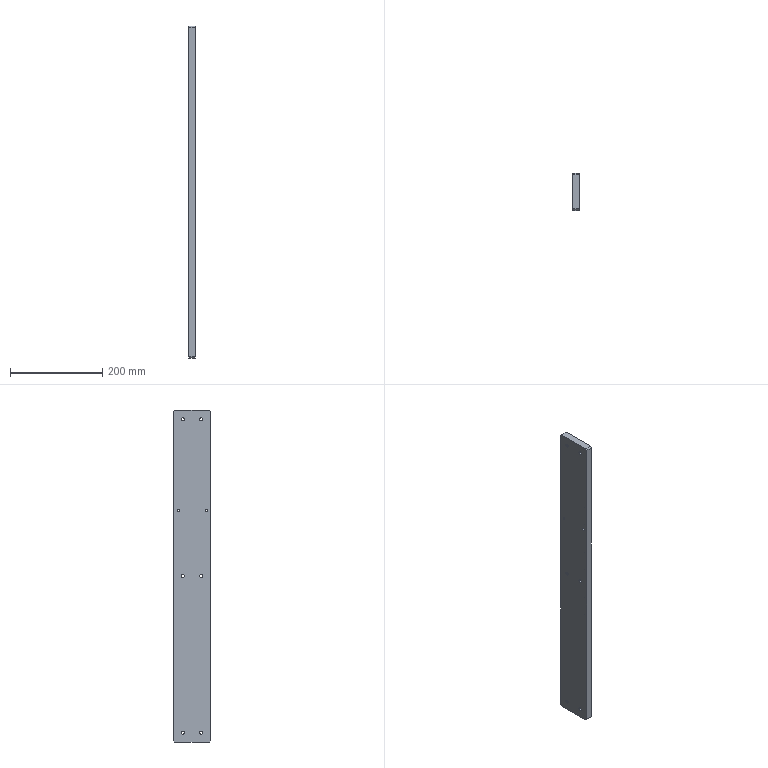Part | SolidWorks | features HoleWzd 7, Chamfer 1, Extrusion 1 | 1 solid | 118 faces | box 15 x 80 x 720 mm | volume 856123 mm3 | cylinder 60 | cone 48 | plane 10 | commonest cylinder face diameters 5 x24 4.2 x16 6.8 x12 6 x8